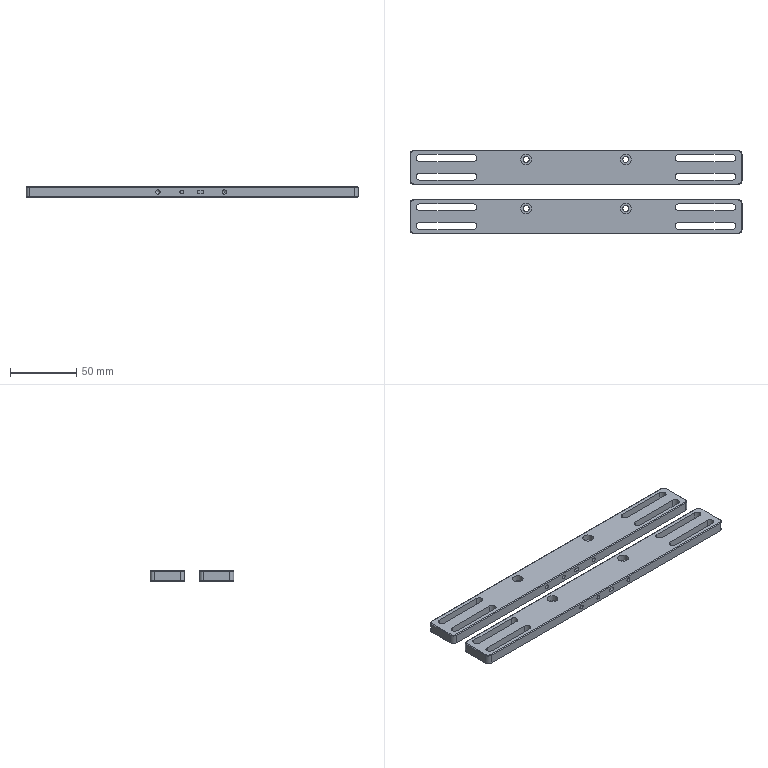Part | 2 solids | 118 faces | box 250 x 63 x 8 mm | volume 85983 mm3 | plane 56 | cylinder 42 | cone 20 | commonest cylinder face diameters 5.5 x16 6 x8 3 x6 3.242 x4 4.5 x4 8 x4